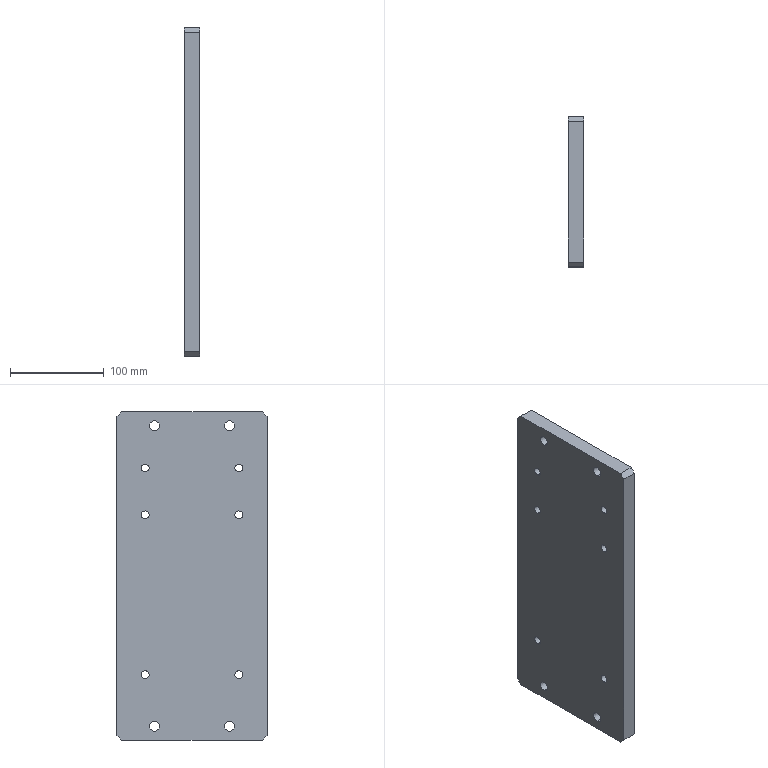Part | SolidWorks | features HoleWzd 2, Chamfer 1, Extrusion 1 | 1 solid | 30 faces | box 16 x 160 x 350 mm | volume 884211 mm3 | cylinder 20 | plane 10 | commonest cylinder face diameters 8.5 x12 10.5 x8
STEP:
#1=CARTESIAN_POINT('',(16.,40.,-165.25));
#2=VERTEX_POINT('',#1);
#3=CARTESIAN_POINT('',(16.,40.,-154.75));
#4=VERTEX_POINT('',#3);
#5=CARTESIAN_POINT('',(16.,40.,-160.));
#6=DIRECTION('',(-1.,0.,0.));
#7=DIRECTION('',(0.,0.,1.));
#8=AXIS2_PLACEMENT_3D('',#5,#6,#7);
#9=CIRCLE('',#8,5.25);
#10=EDGE_CURVE('',#2,#4,#9,.T.);
#11=ORIENTED_EDGE('',*,*,#10,.F.);
#12=CARTESIAN_POINT('',(0.,40.,-165.25));
#13=VERTEX_POINT('',#12);
#14=CARTESIAN_POINT('',(0.,40.,-165.25));
#15=DIRECTION('',(-1.,0.,0.));
#16=VECTOR('',#15,1000.);
#17=LINE('',#14,#16);
#18=EDGE_CURVE('',#2,#13,#17,.T.);
#19=ORIENTED_EDGE('',*,*,#18,.T.);
#20=CARTESIAN_POINT('',(0.,40.,-154.75));
#21=VERTEX_POINT('',#20);
#22=CARTESIAN_POINT('',(0.,40.,-160.));
#23=DIRECTION('',(-1.,0.,0.));
#24=DIRECTION('',(0.,0.,1.));
#25=AXIS2_PLACEMENT_3D('',#22,#23,#24);
#26=CIRCLE('',#25,5.25);
#27=EDGE_CURVE('',#13,#21,#26,.T.);
#28=ORIENTED_EDGE('',*,*,#27,.T.);
#29=CARTESIAN_POINT('',(0.,40.,-154.75));
#30=DIRECTION('',(-1.,0.,0.));
#31=VECTOR('',#30,1000.);
#32=LINE('',#29,#31);
#33=EDGE_CURVE('',#4,#21,#32,.T.);
#34=ORIENTED_EDGE('',*,*,#33,.F.);
#35=EDGE_LOOP('',(#11,#19,#28,#34));
#36=FACE_OUTER_BOUND('',#35,.T.);
#37=CARTESIAN_POINT('',(0.,40.,-160.));
#38=DIRECTION('',(-1.,0.,0.));
#39=DIRECTION('',(0.,0.,1.));
#40=AXIS2_PLACEMENT_3D('',#37,#38,#39);
#41=CYLINDRICAL_SURFACE('',#40,5.25);
#42=ADVANCED_FACE('',(#36),#41,.F.);
#43=CARTESIAN_POINT('',(16.,-40.,-165.25));
#44=VERTEX_POINT('',#43);
#45=CARTESIAN_POINT('',(16.,-40.,-154.75));
#46=VERTEX_POINT('',#45);
#47=CARTESIAN_POINT('',(16.,-40.,-160.));
#48=DIRECTION('',(-1.,0.,0.));
#49=DIRECTION('',(0.,0.,1.));
#50=AXIS2_PLACEMENT_3D('',#47,#48,#49);
#51=CIRCLE('',#50,5.25);
#52=EDGE_CURVE('',#44,#46,#51,.T.);
#53=ORIENTED_EDGE('',*,*,#52,.F.);
#54=CARTESIAN_POINT('',(0.,-40.,-165.25));
#55=VERTEX_POINT('',#54);
#56=CARTESIAN_POINT('',(0.,-40.,-165.25));
#57=DIRECTION('',(-1.,0.,0.));
#58=VECTOR('',#57,1000.);
#59=LINE('',#56,#58);
#60=EDGE_CURVE('',#44,#55,#59,.T.);
#61=ORIENTED_EDGE('',*,*,#60,.T.);
#62=CARTESIAN_POINT('',(0.,-40.,-154.75));
#63=VERTEX_POINT('',#62);
#64=CARTESIAN_POINT('',(0.,-40.,-160.));
#65=DIRECTION('',(-1.,0.,0.));
#66=DIRECTION('',(0.,0.,1.));
#67=AXIS2_PLACEMENT_3D('',#64,#65,#66);
#68=CIRCLE('',#67,5.25);
#69=EDGE_CURVE('',#55,#63,#68,.T.);
#70=ORIENTED_EDGE('',*,*,#69,.T.);
#71=CARTESIAN_POINT('',(0.,-40.,-154.75));
#72=DIRECTION('',(-1.,0.,0.));
#73=VECTOR('',#72,1000.);
#74=LINE('',#71,#73);
#75=EDGE_CURVE('',#46,#63,#74,.T.);
#76=ORIENTED_EDGE('',*,*,#75,.F.);
#77=EDGE_LOOP('',(#53,#61,#70,#76));
#78=FACE_OUTER_BOUND('',#77,.T.);
#79=CARTESIAN_POINT('',(0.,-40.,-160.));
#80=DIRECTION('',(-1.,0.,0.));
#81=DIRECTION('',(0.,0.,1.));
#82=AXIS2_PLACEMENT_3D('',#79,#80,#81);
#83=CYLINDRICAL_SURFACE('',#82,5.25);
#84=ADVANCED_FACE('',(#78),#83,.F.);
#85=CARTESIAN_POINT('',(16.,40.,154.75));
#86=VERTEX_POINT('',#85);
#87=CARTESIAN_POINT('',(16.,40.,165.25));
#88=VERTEX_POINT('',#87);
#89=CARTESIAN_POINT('',(16.,40.,160.));
#90=DIRECTION('',(-1.,0.,0.));
#91=DIRECTION('',(0.,0.,1.));
#92=AXIS2_PLACEMENT_3D('',#89,#90,#91);
#93=CIRCLE('',#92,5.25);
#94=EDGE_CURVE('',#86,#88,#93,.T.);
#95=ORIENTED_EDGE('',*,*,#94,.F.);
#96=CARTESIAN_POINT('',(0.,40.,154.75));
#97=VERTEX_POINT('',#96);
#98=CARTESIAN_POINT('',(0.,40.,154.75));
#99=DIRECTION('',(-1.,0.,0.));
#100=VECTOR('',#99,1000.);
#101=LINE('',#98,#100);
#102=EDGE_CURVE('',#86,#97,#101,.T.);
#103=ORIENTED_EDGE('',*,*,#102,.T.);
#104=CARTESIAN_POINT('',(0.,40.,165.25));
#105=VERTEX_POINT('',#104);
#106=CARTESIAN_POINT('',(0.,40.,160.));
#107=DIRECTION('',(-1.,0.,0.));
#108=DIRECTION('',(0.,0.,1.));
#109=AXIS2_PLACEMENT_3D('',#106,#107,#108);
#110=CIRCLE('',#109,5.25);
#111=EDGE_CURVE('',#97,#105,#110,.T.);
#112=ORIENTED_EDGE('',*,*,#111,.T.);
#113=CARTESIAN_POINT('',(0.,40.,165.25));
#114=DIRECTION('',(-1.,0.,0.));
#115=VECTOR('',#114,1000.);
#116=LINE('',#113,#115);
#117=EDGE_CURVE('',#88,#105,#116,.T.);
#118=ORIENTED_EDGE('',*,*,#117,.F.);
#119=EDGE_LOOP('',(#95,#103,#112,#118));
#120=FACE_OUTER_BOUND('',#119,.T.);
#121=CARTESIAN_POINT('',(0.,40.,160.));
#122=DIRECTION('',(-1.,0.,0.));
#123=DIRECTION('',(0.,0.,1.));
#124=AXIS2_PLACEMENT_3D('',#121,#122,#123);
#125=CYLINDRICAL_SURFACE('',#124,5.25);
#126=ADVANCED_FACE('',(#120),#125,.F.);
#127=CARTESIAN_POINT('',(16.,-40.,154.75));
#128=VERTEX_POINT('',#127);
#129=CARTESIAN_POINT('',(16.,-40.,165.25));
#130=VERTEX_POINT('',#129);
#131=CARTESIAN_POINT('',(16.,-40.,160.));
#132=DIRECTION('',(-1.,0.,0.));
#133=DIRECTION('',(0.,0.,1.));
#134=AXIS2_PLACEMENT_3D('',#131,#132,#133);
#135=CIRCLE('',#134,5.25);
#136=EDGE_CURVE('',#128,#130,#135,.T.);
#137=ORIENTED_EDGE('',*,*,#136,.F.);
#138=CARTESIAN_POINT('',(0.,-40.,154.75));
#139=VERTEX_POINT('',#138);
#140=CARTESIAN_POINT('',(0.,-40.,154.75));
#141=DIRECTION('',(-1.,0.,0.));
#142=VECTOR('',#141,1000.);
#143=LINE('',#140,#142);
#144=EDGE_CURVE('',#128,#139,#143,.T.);
#145=ORIENTED_EDGE('',*,*,#144,.T.);
#146=CARTESIAN_POINT('',(0.,-40.,165.25));
#147=VERTEX_POINT('',#146);
#148=CARTESIAN_POINT('',(0.,-40.,160.));
#149=DIRECTION('',(-1.,0.,0.));
#150=DIRECTION('',(0.,0.,1.));
#151=AXIS2_PLACEMENT_3D('',#148,#149,#150);
#152=CIRCLE('',#151,5.25);
#153=EDGE_CURVE('',#139,#147,#152,.T.);
#154=ORIENTED_EDGE('',*,*,#153,.T.);
#155=CARTESIAN_POINT('',(0.,-40.,165.25));
#156=DIRECTION('',(-1.,0.,0.));
#157=VECTOR('',#156,1000.);
#158=LINE('',#155,#157);
#159=EDGE_CURVE('',#130,#147,#158,.T.);
#160=ORIENTED_EDGE('',*,*,#159,.F.);
#161=EDGE_LOOP('',(#137,#145,#154,#160));
#162=FACE_OUTER_BOUND('',#161,.T.);
#163=CARTESIAN_POINT('',(0.,-40.,160.));
#164=DIRECTION('',(-1.,0.,0.));
#165=DIRECTION('',(0.,0.,1.));
#166=AXIS2_PLACEMENT_3D('',#163,#164,#165);
#167=CYLINDRICAL_SURFACE('',#166,5.25);
#168=ADVANCED_FACE('',(#162),#167,.F.);
#169=CARTESIAN_POINT('',(0.,50.,119.25));
#170=VERTEX_POINT('',#169);
#171=CARTESIAN_POINT('',(0.,50.,110.75));
#172=VERTEX_POINT('',#171);
#173=CARTESIAN_POINT('',(0.,50.,115.));
#174=DIRECTION('',(1.,0.,0.));
#175=DIRECTION('',(0.,0.,-1.));
#176=AXIS2_PLACEMENT_3D('',#173,#174,#175);
#177=CIRCLE('',#176,4.25);
#178=EDGE_CURVE('',#170,#172,#177,.T.);
#179=ORIENTED_EDGE('',*,*,#178,.F.);
#180=CARTESIAN_POINT('',(16.,50.,119.25));
#181=VERTEX_POINT('',#180);
#182=CARTESIAN_POINT('',(16.,50.,119.25));
#183=DIRECTION('',(1.,0.,0.));
#184=VECTOR('',#183,1000.);
#185=LINE('',#182,#184);
#186=EDGE_CURVE('',#170,#181,#185,.T.);
#187=ORIENTED_EDGE('',*,*,#186,.T.);
#188=CARTESIAN_POINT('',(16.,50.,110.75));
#189=VERTEX_POINT('',#188);
#190=CARTESIAN_POINT('',(16.,50.,115.));
#191=DIRECTION('',(1.,0.,0.));
#192=DIRECTION('',(0.,0.,-1.));
#193=AXIS2_PLACEMENT_3D('',#190,#191,#192);
#194=CIRCLE('',#193,4.25);
#195=EDGE_CURVE('',#181,#189,#194,.T.);
#196=ORIENTED_EDGE('',*,*,#195,.T.);
#197=CARTESIAN_POINT('',(16.,50.,110.75));
#198=DIRECTION('',(1.,0.,0.));
#199=VECTOR('',#198,1000.);
#200=LINE('',#197,#199);
#201=EDGE_CURVE('',#172,#189,#200,.T.);
#202=ORIENTED_EDGE('',*,*,#201,.F.);
#203=EDGE_LOOP('',(#179,#187,#196,#202));
#204=FACE_OUTER_BOUND('',#203,.T.);
#205=CARTESIAN_POINT('',(16.,50.,115.));
#206=DIRECTION('',(1.,0.,0.));
#207=DIRECTION('',(0.,0.,-1.));
#208=AXIS2_PLACEMENT_3D('',#205,#206,#207);
#209=CYLINDRICAL_SURFACE('',#208,4.25);
#210=ADVANCED_FACE('',(#204),#209,.F.);
#211=CARTESIAN_POINT('',(0.,-50.,119.25));
#212=VERTEX_POINT('',#211);
#213=CARTESIAN_POINT('',(0.,-50.,110.75));
#214=VERTEX_POINT('',#213);
#215=CARTESIAN_POINT('',(0.,-50.,115.));
#216=DIRECTION('',(1.,0.,0.));
#217=DIRECTION('',(0.,0.,-1.));
#218=AXIS2_PLACEMENT_3D('',#215,#216,#217);
#219=CIRCLE('',#218,4.25);
#220=EDGE_CURVE('',#212,#214,#219,.T.);
#221=ORIENTED_EDGE('',*,*,#220,.F.);
#222=CARTESIAN_POINT('',(16.,-50.,119.25));
#223=VERTEX_POINT('',#222);
#224=CARTESIAN_POINT('',(16.,-50.,119.25));
#225=DIRECTION('',(1.,0.,0.));
#226=VECTOR('',#225,1000.);
#227=LINE('',#224,#226);
#228=EDGE_CURVE('',#212,#223,#227,.T.);
#229=ORIENTED_EDGE('',*,*,#228,.T.);
#230=CARTESIAN_POINT('',(16.,-50.,110.75));
#231=VERTEX_POINT('',#230);
#232=CARTESIAN_POINT('',(16.,-50.,115.));
#233=DIRECTION('',(1.,0.,0.));
#234=DIRECTION('',(0.,0.,-1.));
#235=AXIS2_PLACEMENT_3D('',#232,#233,#234);
#236=CIRCLE('',#235,4.25);
#237=EDGE_CURVE('',#223,#231,#236,.T.);
#238=ORIENTED_EDGE('',*,*,#237,.T.);
#239=CARTESIAN_POINT('',(16.,-50.,110.75));
#240=DIRECTION('',(1.,0.,0.));
#241=VECTOR('',#240,1000.);
#242=LINE('',#239,#241);
#243=EDGE_CURVE('',#214,#231,#242,.T.);
#244=ORIENTED_EDGE('',*,*,#243,.F.);
#245=EDGE_LOOP('',(#221,#229,#238,#244));
#246=FACE_OUTER_BOUND('',#245,.T.);
#247=CARTESIAN_POINT('',(16.,-50.,115.));
#248=DIRECTION('',(1.,0.,0.));
#249=DIRECTION('',(0.,0.,-1.));
#250=AXIS2_PLACEMENT_3D('',#247,#248,#249);
#251=CYLINDRICAL_SURFACE('',#250,4.25);
#252=ADVANCED_FACE('',(#246),#251,.F.);
#253=CARTESIAN_POINT('',(0.,50.,-100.75));
#254=VERTEX_POINT('',#253);
#255=CARTESIAN_POINT('',(0.,50.,-109.25));
#256=VERTEX_POINT('',#255);
#257=CARTESIAN_POINT('',(0.,50.,-105.));
#258=DIRECTION('',(1.,0.,0.));
#259=DIRECTION('',(0.,0.,-1.));
#260=AXIS2_PLACEMENT_3D('',#257,#258,#259);
#261=CIRCLE('',#260,4.25);
#262=EDGE_CURVE('',#254,#256,#261,.T.);
#263=ORIENTED_EDGE('',*,*,#262,.F.);
#264=CARTESIAN_POINT('',(16.,50.,-100.75));
#265=VERTEX_POINT('',#264);
#266=CARTESIAN_POINT('',(16.,50.,-100.75));
#267=DIRECTION('',(1.,0.,0.));
#268=VECTOR('',#267,1000.);
#269=LINE('',#266,#268);
#270=EDGE_CURVE('',#254,#265,#269,.T.);
#271=ORIENTED_EDGE('',*,*,#270,.T.);
#272=CARTESIAN_POINT('',(16.,50.,-109.25));
#273=VERTEX_POINT('',#272);
#274=CARTESIAN_POINT('',(16.,50.,-105.));
#275=DIRECTION('',(1.,0.,0.));
#276=DIRECTION('',(0.,0.,-1.));
#277=AXIS2_PLACEMENT_3D('',#274,#275,#276);
#278=CIRCLE('',#277,4.25);
#279=EDGE_CURVE('',#265,#273,#278,.T.);
#280=ORIENTED_EDGE('',*,*,#279,.T.);
#281=CARTESIAN_POINT('',(16.,50.,-109.25));
#282=DIRECTION('',(1.,0.,0.));
#283=VECTOR('',#282,1000.);
#284=LINE('',#281,#283);
#285=EDGE_CURVE('',#256,#273,#284,.T.);
#286=ORIENTED_EDGE('',*,*,#285,.F.);
#287=EDGE_LOOP('',(#263,#271,#280,#286));
#288=FACE_OUTER_BOUND('',#287,.T.);
#289=CARTESIAN_POINT('',(16.,50.,-105.));
#290=DIRECTION('',(1.,0.,0.));
#291=DIRECTION('',(0.,0.,-1.));
#292=AXIS2_PLACEMENT_3D('',#289,#290,#291);
#293=CYLINDRICAL_SURFACE('',#292,4.25);
#294=ADVANCED_FACE('',(#288),#293,.F.);
#295=CARTESIAN_POINT('',(0.,-50.,-100.75));
#296=VERTEX_POINT('',#295);
#297=CARTESIAN_POINT('',(0.,-50.,-109.25));
#298=VERTEX_POINT('',#297);
#299=CARTESIAN_POINT('',(0.,-50.,-105.));
#300=DIRECTION('',(1.,0.,0.));
#301=DIRECTION('',(0.,0.,-1.));
#302=AXIS2_PLACEMENT_3D('',#299,#300,#301);
#303=CIRCLE('',#302,4.25);
#304=EDGE_CURVE('',#296,#298,#303,.T.);
#305=ORIENTED_EDGE('',*,*,#304,.F.);
#306=CARTESIAN_POINT('',(16.,-50.,-100.75));
#307=VERTEX_POINT('',#306);
#308=CARTESIAN_POINT('',(16.,-50.,-100.75));
#309=DIRECTION('',(1.,0.,0.));
#310=VECTOR('',#309,1000.);
#311=LINE('',#308,#310);
#312=EDGE_CURVE('',#296,#307,#311,.T.);
#313=ORIENTED_EDGE('',*,*,#312,.T.);
#314=CARTESIAN_POINT('',(16.,-50.,-109.25));
#315=VERTEX_POINT('',#314);
#316=CARTESIAN_POINT('',(16.,-50.,-105.));
#317=DIRECTION('',(1.,0.,0.));
#318=DIRECTION('',(0.,0.,-1.));
#319=AXIS2_PLACEMENT_3D('',#316,#317,#318);
#320=CIRCLE('',#319,4.25);
#321=EDGE_CURVE('',#307,#315,#320,.T.);
#322=ORIENTED_EDGE('',*,*,#321,.T.);
#323=CARTESIAN_POINT('',(16.,-50.,-109.25));
#324=DIRECTION('',(1.,0.,0.));
#325=VECTOR('',#324,1000.);
#326=LINE('',#323,#325);
#327=EDGE_CURVE('',#298,#315,#326,.T.);
#328=ORIENTED_EDGE('',*,*,#327,.F.);
#329=EDGE_LOOP('',(#305,#313,#322,#328));
#330=FACE_OUTER_BOUND('',#329,.T.);
#331=CARTESIAN_POINT('',(16.,-50.,-105.));
#332=DIRECTION('',(1.,0.,0.));
#333=DIRECTION('',(0.,0.,-1.));
#334=AXIS2_PLACEMENT_3D('',#331,#332,#333);
#335=CYLINDRICAL_SURFACE('',#334,4.25);
#336=ADVANCED_FACE('',(#330),#335,.F.);
#337=CARTESIAN_POINT('',(0.,50.,69.25));
#338=VERTEX_POINT('',#337);
#339=CARTESIAN_POINT('',(0.,50.,60.75));
#340=VERTEX_POINT('',#339);
#341=CARTESIAN_POINT('',(0.,50.,65.));
#342=DIRECTION('',(1.,0.,0.));
#343=DIRECTION('',(0.,0.,-1.));
#344=AXIS2_PLACEMENT_3D('',#341,#342,#343);
#345=CIRCLE('',#344,4.25);
#346=EDGE_CURVE('',#338,#340,#345,.T.);
#347=ORIENTED_EDGE('',*,*,#346,.F.);
#348=CARTESIAN_POINT('',(16.,50.,69.25));
#349=VERTEX_POINT('',#348);
#350=CARTESIAN_POINT('',(16.,50.,69.25));
#351=DIRECTION('',(1.,0.,0.));
#352=VECTOR('',#351,1000.);
#353=LINE('',#350,#352);
#354=EDGE_CURVE('',#338,#349,#353,.T.);
#355=ORIENTED_EDGE('',*,*,#354,.T.);
#356=CARTESIAN_POINT('',(16.,50.,60.75));
#357=VERTEX_POINT('',#356);
#358=CARTESIAN_POINT('',(16.,50.,65.));
#359=DIRECTION('',(1.,0.,0.));
#360=DIRECTION('',(0.,0.,-1.));
#361=AXIS2_PLACEMENT_3D('',#358,#359,#360);
#362=CIRCLE('',#361,4.25);
#363=EDGE_CURVE('',#349,#357,#362,.T.);
#364=ORIENTED_EDGE('',*,*,#363,.T.);
#365=CARTESIAN_POINT('',(16.,50.,60.75));
#366=DIRECTION('',(1.,0.,0.));
#367=VECTOR('',#366,1000.);
#368=LINE('',#365,#367);
#369=EDGE_CURVE('',#340,#357,#368,.T.);
#370=ORIENTED_EDGE('',*,*,#369,.F.);
#371=EDGE_LOOP('',(#347,#355,#364,#370));
#372=FACE_OUTER_BOUND('',#371,.T.);
#373=CARTESIAN_POINT('',(16.,50.,65.));
#374=DIRECTION('',(1.,0.,0.));
#375=DIRECTION('',(0.,0.,-1.));
#376=AXIS2_PLACEMENT_3D('',#373,#374,#375);
#377=CYLINDRICAL_SURFACE('',#376,4.25);
#378=ADVANCED_FACE('',(#372),#377,.F.);
#379=CARTESIAN_POINT('',(0.,-50.,69.25));
#380=VERTEX_POINT('',#379);
#381=CARTESIAN_POINT('',(0.,-50.,60.75));
#382=VERTEX_POINT('',#381);
#383=CARTESIAN_POINT('',(0.,-50.,65.));
#384=DIRECTION('',(1.,0.,0.));
#385=DIRECTION('',(0.,0.,-1.));
#386=AXIS2_PLACEMENT_3D('',#383,#384,#385);
#387=CIRCLE('',#386,4.25);
#388=EDGE_CURVE('',#380,#382,#387,.T.);
#389=ORIENTED_EDGE('',*,*,#388,.F.);
#390=CARTESIAN_POINT('',(16.,-50.,69.25));
#391=VERTEX_POINT('',#390);
#392=CARTESIAN_POINT('',(16.,-50.,69.25));
#393=DIRECTION('',(1.,0.,0.));
#394=VECTOR('',#393,1000.);
#395=LINE('',#392,#394);
#396=EDGE_CURVE('',#380,#391,#395,.T.);
#397=ORIENTED_EDGE('',*,*,#396,.T.);
#398=CARTESIAN_POINT('',(16.,-50.,60.75));
#399=VERTEX_POINT('',#398);
#400=CARTESIAN_POINT('',(16.,-50.,65.));
#401=DIRECTION('',(1.,0.,0.));
#402=DIRECTION('',(0.,0.,-1.));
#403=AXIS2_PLACEMENT_3D('',#400,#401,#402);
#404=CIRCLE('',#403,4.25);
#405=EDGE_CURVE('',#391,#399,#404,.T.);
#406=ORIENTED_EDGE('',*,*,#405,.T.);
#407=CARTESIAN_POINT('',(16.,-50.,60.75));
#408=DIRECTION('',(1.,0.,0.));
#409=VECTOR('',#408,1000.);
#410=LINE('',#407,#409);
#411=EDGE_CURVE('',#382,#399,#410,.T.);
#412=ORIENTED_EDGE('',*,*,#411,.F.);
#413=EDGE_LOOP('',(#389,#397,#406,#412));
#414=FACE_OUTER_BOUND('',#413,.T.);
#415=CARTESIAN_POINT('',(16.,-50.,65.));
#416=DIRECTION('',(1.,0.,0.));
#417=DIRECTION('',(0.,0.,-1.));
#418=AXIS2_PLACEMENT_3D('',#415,#416,#417);
#419=CYLINDRICAL_SURFACE('',#418,4.25);
#420=ADVANCED_FACE('',(#414),#419,.F.);
#421=CARTESIAN_POINT('',(0.,40.,-160.));
#422=DIRECTION('',(-1.,0.,0.));
#423=DIRECTION('',(0.,0.,1.));
#424=AXIS2_PLACEMENT_3D('',#421,#422,#423);
#425=CIRCLE('',#424,5.25);
#426=EDGE_CURVE('',#21,#13,#425,.T.);
#427=ORIENTED_EDGE('',*,*,#426,.F.);
#428=ORIENTED_EDGE('',*,*,#27,.F.);
#429=EDGE_LOOP('',(#427,#428));
#430=FACE_BOUND('',#429,.T.);
#431=CARTESIAN_POINT('',(0.,-40.,-160.));
#432=DIRECTION('',(-1.,0.,0.));
#433=DIRECTION('',(0.,0.,1.));
#434=AXIS2_PLACEMENT_3D('',#431,#432,#433);
#435=CIRCLE('',#434,5.25);
#436=EDGE_CURVE('',#63,#55,#435,.T.);
#437=ORIENTED_EDGE('',*,*,#436,.F.);
#438=ORIENTED_EDGE('',*,*,#69,.F.);
#439=EDGE_LOOP('',(#437,#438));
#440=FACE_BOUND('',#439,.T.);
#441=CARTESIAN_POINT('',(0.,-40.,160.));
#442=DIRECTION('',(-1.,0.,0.));
#443=DIRECTION('',(0.,0.,1.));
#444=AXIS2_PLACEMENT_3D('',#441,#442,#443);
#445=CIRCLE('',#444,5.25);
#446=EDGE_CURVE('',#147,#139,#445,.T.);
#447=ORIENTED_EDGE('',*,*,#446,.F.);
#448=ORIENTED_EDGE('',*,*,#153,.F.);
#449=EDGE_LOOP('',(#447,#448));
#450=FACE_BOUND('',#449,.T.);
#451=CARTESIAN_POINT('',(0.,50.,115.));
#452=DIRECTION('',(1.,0.,0.));
#453=DIRECTION('',(0.,0.,-1.));
#454=AXIS2_PLACEMENT_3D('',#451,#452,#453);
#455=CIRCLE('',#454,4.25);
#456=EDGE_CURVE('',#172,#170,#455,.T.);
#457=ORIENTED_EDGE('',*,*,#456,.T.);
#458=ORIENTED_EDGE('',*,*,#178,.T.);
#459=EDGE_LOOP('',(#457,#458));
#460=FACE_BOUND('',#459,.T.);
#461=CARTESIAN_POINT('',(0.,-50.,115.));
#462=DIRECTION('',(1.,0.,0.));
#463=DIRECTION('',(0.,0.,-1.));
#464=AXIS2_PLACEMENT_3D('',#461,#462,#463);
#465=CIRCLE('',#464,4.25);
#466=EDGE_CURVE('',#214,#212,#465,.T.);
#467=ORIENTED_EDGE('',*,*,#466,.T.);
#468=ORIENTED_EDGE('',*,*,#220,.T.);
#469=EDGE_LOOP('',(#467,#468));
#470=FACE_BOUND('',#469,.T.);
#471=CARTESIAN_POINT('',(0.,50.,-105.));
#472=DIRECTION('',(1.,0.,0.));
#473=DIRECTION('',(0.,0.,-1.));
#474=AXIS2_PLACEMENT_3D('',#471,#472,#473);
#475=CIRCLE('',#474,4.25);
#476=EDGE_CURVE('',#256,#254,#475,.T.);
#477=ORIENTED_EDGE('',*,*,#476,.T.);
#478=ORIENTED_EDGE('',*,*,#262,.T.);
#479=EDGE_LOOP('',(#477,#478));
#480=FACE_BOUND('',#479,.T.);
#481=CARTESIAN_POINT('',(0.,-50.,-105.));
#482=DIRECTION('',(1.,0.,0.));
#483=DIRECTION('',(0.,0.,-1.));
#484=AXIS2_PLACEMENT_3D('',#481,#482,#483);
#485=CIRCLE('',#484,4.25);
#486=EDGE_CURVE('',#298,#296,#485,.T.);
#487=ORIENTED_EDGE('',*,*,#486,.T.);
#488=ORIENTED_EDGE('',*,*,#304,.T.);
#489=EDGE_LOOP('',(#487,#488));
#490=FACE_BOUND('',#489,.T.);
#491=CARTESIAN_POINT('',(0.,50.,65.));
#492=DIRECTION('',(1.,0.,0.));
#493=DIRECTION('',(0.,0.,-1.));
#494=AXIS2_PLACEMENT_3D('',#491,#492,#493);
#495=CIRCLE('',#494,4.25);
#496=EDGE_CURVE('',#340,#338,#495,.T.);
#497=ORIENTED_EDGE('',*,*,#496,.T.);
#498=ORIENTED_EDGE('',*,*,#346,.T.);
#499=EDGE_LOOP('',(#497,#498));
#500=FACE_BOUND('',#499,.T.);
#501=CARTESIAN_POINT('',(0.,-50.,65.));
#502=DIRECTION('',(1.,0.,0.));
#503=DIRECTION('',(0.,0.,-1.));
#504=AXIS2_PLACEMENT_3D('',#501,#502,#503);
#505=CIRCLE('',#504,4.25);
#506=EDGE_CURVE('',#382,#380,#505,.T.);
#507=ORIENTED_EDGE('',*,*,#506,.T.);
#508=ORIENTED_EDGE('',*,*,#388,.T.);
#509=EDGE_LOOP('',(#507,#508));
#510=FACE_BOUND('',#509,.T.);
#511=CARTESIAN_POINT('',(0.,75.,175.));
#512=VERTEX_POINT('',#511);
#513=CARTESIAN_POINT('',(0.,-75.,175.));
#514=VERTEX_POINT('',#513);
#515=CARTESIAN_POINT('',(0.,80.,175.));
#516=DIRECTION('',(0.,-1.,0.));
#517=VECTOR('',#516,1000.);
#518=LINE('',#515,#517);
#519=EDGE_CURVE('',#512,#514,#518,.T.);
#520=ORIENTED_EDGE('',*,*,#519,.F.);
#521=CARTESIAN_POINT('',(0.,80.,170.));
#522=VERTEX_POINT('',#521);
#523=CARTESIAN_POINT('',(0.,75.,175.));
#524=DIRECTION('',(0.,0.7071,-0.7071));
#525=VECTOR('',#524,1000.);
#526=LINE('',#523,#525);
#527=EDGE_CURVE('',#512,#522,#526,.T.);
#528=ORIENTED_EDGE('',*,*,#527,.T.);
#529=CARTESIAN_POINT('',(0.,80.,-170.));
#530=VERTEX_POINT('',#529);
#531=CARTESIAN_POINT('',(0.,80.,175.));
#532=DIRECTION('',(0.,0.,1.));
#533=VECTOR('',#532,1000.);
#534=LINE('',#531,#533);
#535=EDGE_CURVE('',#530,#522,#534,.T.);
#536=ORIENTED_EDGE('',*,*,#535,.F.);
#537=CARTESIAN_POINT('',(0.,75.,-175.));
#538=VERTEX_POINT('',#537);
#539=CARTESIAN_POINT('',(0.,80.,-170.));
#540=DIRECTION('',(0.,-0.7071,-0.7071));
#541=VECTOR('',#540,1000.);
#542=LINE('',#539,#541);
#543=EDGE_CURVE('',#530,#538,#542,.T.);
#544=ORIENTED_EDGE('',*,*,#543,.T.);
#545=CARTESIAN_POINT('',(0.,-75.,-175.));
#546=VERTEX_POINT('',#545);
#547=CARTESIAN_POINT('',(0.,80.,-175.));
#548=DIRECTION('',(0.,1.,0.));
#549=VECTOR('',#548,1000.);
#550=LINE('',#547,#549);
#551=EDGE_CURVE('',#546,#538,#550,.T.);
#552=ORIENTED_EDGE('',*,*,#551,.F.);
#553=CARTESIAN_POINT('',(0.,-80.,-170.));
#554=VERTEX_POINT('',#553);
#555=CARTESIAN_POINT('',(0.,-75.,-175.));
#556=DIRECTION('',(0.,-0.7071,0.7071));
#557=VECTOR('',#556,1000.);
#558=LINE('',#555,#557);
#559=EDGE_CURVE('',#546,#554,#558,.T.);
#560=ORIENTED_EDGE('',*,*,#559,.T.);
#561=CARTESIAN_POINT('',(0.,-80.,170.));
#562=VERTEX_POINT('',#561);
#563=CARTESIAN_POINT('',(0.,-80.,175.));
#564=DIRECTION('',(0.,0.,-1.));
#565=VECTOR('',#564,1000.);
#566=LINE('',#563,#565);
#567=EDGE_CURVE('',#562,#554,#566,.T.);
#568=ORIENTED_EDGE('',*,*,#567,.F.);
#569=CARTESIAN_POINT('',(0.,-80.,170.));
#570=DIRECTION('',(0.,0.7071,0.7071));
#571=VECTOR('',#570,1000.);
#572=LINE('',#569,#571);
#573=EDGE_CURVE('',#562,#514,#572,.T.);
#574=ORIENTED_EDGE('',*,*,#573,.T.);
#575=EDGE_LOOP('',(#520,#528,#536,#544,#552,#560,#568,#574));
#576=FACE_OUTER_BOUND('',#575,.T.);
#577=CARTESIAN_POINT('',(0.,40.,160.));
#578=DIRECTION('',(-1.,0.,0.));
#579=DIRECTION('',(0.,0.,1.));
#580=AXIS2_PLACEMENT_3D('',#577,#578,#579);
#581=CIRCLE('',#580,5.25);
#582=EDGE_CURVE('',#105,#97,#581,.T.);
#583=ORIENTED_EDGE('',*,*,#582,.F.);
#584=ORIENTED_EDGE('',*,*,#111,.F.);
#585=EDGE_LOOP('',(#583,#584));
#586=FACE_BOUND('',#585,.T.);
#587=CARTESIAN_POINT('',(0.,0.,0.));
#588=DIRECTION('',(1.,0.,0.));
#589=DIRECTION('',(0.,0.,-1.));
#590=AXIS2_PLACEMENT_3D('',#587,#588,#589);
#591=PLANE('',#590);
#592=ADVANCED_FACE('',(#430,#440,#450,#460,#470,#480,#490,#500,#510,#576,#586),#591,.F.);
#593=ORIENTED_EDGE('',*,*,#551,.T.);
#594=CARTESIAN_POINT('',(16.,75.,-175.));
#595=VERTEX_POINT('',#594);
#596=CARTESIAN_POINT('',(16.,75.,-175.));
#597=DIRECTION('',(1.,0.,0.));
#598=VECTOR('',#597,1000.);
#599=LINE('',#596,#598);
#600=EDGE_CURVE('',#538,#595,#599,.T.);
#601=ORIENTED_EDGE('',*,*,#600,.T.);
#602=CARTESIAN_POINT('',(16.,-75.,-175.));
#603=VERTEX_POINT('',#602);
#604=CARTESIAN_POINT('',(16.,80.,-175.));
#605=DIRECTION('',(0.,1.,0.));
#606=VECTOR('',#605,1000.);
#607=LINE('',#604,#606);
#608=EDGE_CURVE('',#603,#595,#607,.T.);
#609=ORIENTED_EDGE('',*,*,#608,.F.);
#610=CARTESIAN_POINT('',(16.,-75.,-175.));
#611=DIRECTION('',(-1.,0.,0.));
#612=VECTOR('',#611,1000.);
#613=LINE('',#610,#612);
#614=EDGE_CURVE('',#603,#546,#613,.T.);
#615=ORIENTED_EDGE('',*,*,#614,.T.);
#616=EDGE_LOOP('',(#593,#601,#609,#615));
#617=FACE_OUTER_BOUND('',#616,.T.);
#618=CARTESIAN_POINT('',(16.,80.,-175.));
#619=DIRECTION('',(0.,0.,1.));
#620=DIRECTION('',(0.,-1.,0.));
#621=AXIS2_PLACEMENT_3D('',#618,#619,#620);
#622=PLANE('',#621);
#623=ADVANCED_FACE('',(#617),#622,.F.);
#624=ORIENTED_EDGE('',*,*,#535,.T.);
#625=CARTESIAN_POINT('',(16.,80.,170.));
#626=VERTEX_POINT('',#625);
#627=CARTESIAN_POINT('',(16.,80.,170.));
#628=DIRECTION('',(1.,0.,0.));
#629=VECTOR('',#628,1000.);
#630=LINE('',#627,#629);
#631=EDGE_CURVE('',#522,#626,#630,.T.);
#632=ORIENTED_EDGE('',*,*,#631,.T.);
#633=CARTESIAN_POINT('',(16.,80.,-170.));
#634=VERTEX_POINT('',#633);
#635=CARTESIAN_POINT('',(16.,80.,175.));
#636=DIRECTION('',(0.,0.,1.));
#637=VECTOR('',#636,1000.);
#638=LINE('',#635,#637);
#639=EDGE_CURVE('',#634,#626,#638,.T.);
#640=ORIENTED_EDGE('',*,*,#639,.F.);
#641=CARTESIAN_POINT('',(16.,80.,-170.));
#642=DIRECTION('',(-1.,0.,0.));
#643=VECTOR('',#642,1000.);
#644=LINE('',#641,#643);
#645=EDGE_CURVE('',#634,#530,#644,.T.);
#646=ORIENTED_EDGE('',*,*,#645,.T.);
#647=EDGE_LOOP('',(#624,#632,#640,#646));
#648=FACE_OUTER_BOUND('',#647,.T.);
#649=CARTESIAN_POINT('',(16.,80.,175.));
#650=DIRECTION('',(0.,-1.,0.));
#651=DIRECTION('',(0.,0.,-1.));
#652=AXIS2_PLACEMENT_3D('',#649,#650,#651);
#653=PLANE('',#652);
#654=ADVANCED_FACE('',(#648),#653,.F.);
#655=CARTESIAN_POINT('',(16.,75.,175.));
#656=VERTEX_POINT('',#655);
#657=CARTESIAN_POINT('',(16.,-75.,175.));
#658=VERTEX_POINT('',#657);
#659=CARTESIAN_POINT('',(16.,80.,175.));
#660=DIRECTION('',(0.,-1.,0.));
#661=VECTOR('',#660,1000.);
#662=LINE('',#659,#661);
#663=EDGE_CURVE('',#656,#658,#662,.T.);
#664=ORIENTED_EDGE('',*,*,#663,.F.);
#665=CARTESIAN_POINT('',(16.,75.,175.));
#666=DIRECTION('',(-1.,0.,0.));
#667=VECTOR('',#666,1000.);
#668=LINE('',#665,#667);
#669=EDGE_CURVE('',#656,#512,#668,.T.);
#670=ORIENTED_EDGE('',*,*,#669,.T.);
#671=ORIENTED_EDGE('',*,*,#519,.T.);
#672=CARTESIAN_POINT('',(16.,-75.,175.));
#673=DIRECTION('',(1.,0.,0.));
#674=VECTOR('',#673,1000.);
#675=LINE('',#672,#674);
#676=EDGE_CURVE('',#514,#658,#675,.T.);
#677=ORIENTED_EDGE('',*,*,#676,.T.);
#678=EDGE_LOOP('',(#664,#670,#671,#677));
#679=FACE_OUTER_BOUND('',#678,.T.);
#680=CARTESIAN_POINT('',(16.,80.,175.));
#681=DIRECTION('',(0.,0.,-1.));
#682=DIRECTION('',(0.,1.,0.));
#683=AXIS2_PLACEMENT_3D('',#680,#681,#682);
#684=PLANE('',#683);
#685=ADVANCED_FACE('',(#679),#684,.F.);
#686=CARTESIAN_POINT('',(16.,-80.,170.));
#687=VERTEX_POINT('',#686);
#688=CARTESIAN_POINT('',(16.,-80.,-170.));
#689=VERTEX_POINT('',#688);
#690=CARTESIAN_POINT('',(16.,-80.,175.));
#691=DIRECTION('',(0.,0.,-1.));
#692=VECTOR('',#691,1000.);
#693=LINE('',#690,#692);
#694=EDGE_CURVE('',#687,#689,#693,.T.);
#695=ORIENTED_EDGE('',*,*,#694,.F.);
#696=CARTESIAN_POINT('',(16.,-80.,170.));
#697=DIRECTION('',(-1.,0.,0.));
#698=VECTOR('',#697,1000.);
#699=LINE('',#696,#698);
#700=EDGE_CURVE('',#687,#562,#699,.T.);
#701=ORIENTED_EDGE('',*,*,#700,.T.);
#702=ORIENTED_EDGE('',*,*,#567,.T.);
#703=CARTESIAN_POINT('',(16.,-80.,-170.));
#704=DIRECTION('',(1.,0.,0.));
#705=VECTOR('',#704,1000.);
#706=LINE('',#703,#705);
#707=EDGE_CURVE('',#554,#689,#706,.T.);
#708=ORIENTED_EDGE('',*,*,#707,.T.);
#709=EDGE_LOOP('',(#695,#701,#702,#708));
#710=FACE_OUTER_BOUND('',#709,.T.);
#711=CARTESIAN_POINT('',(16.,-80.,175.));
#712=DIRECTION('',(0.,1.,0.));
#713=DIRECTION('',(0.,0.,1.));
#714=AXIS2_PLACEMENT_3D('',#711,#712,#713);
#715=PLANE('',#714);
#716=ADVANCED_FACE('',(#710),#715,.F.);
#717=CARTESIAN_POINT('',(16.,40.,-160.));
#718=DIRECTION('',(-1.,0.,0.));
#719=DIRECTION('',(0.,0.,1.));
#720=AXIS2_PLACEMENT_3D('',#717,#718,#719);
#721=CIRCLE('',#720,5.25);
#722=EDGE_CURVE('',#4,#2,#721,.T.);
#723=ORIENTED_EDGE('',*,*,#722,.T.);
#724=ORIENTED_EDGE('',*,*,#10,.T.);
#725=EDGE_LOOP('',(#723,#724));
#726=FACE_BOUND('',#725,.T.);
#727=CARTESIAN_POINT('',(16.,-40.,-160.));
#728=DIRECTION('',(-1.,0.,0.));
#729=DIRECTION('',(0.,0.,1.));
#730=AXIS2_PLACEMENT_3D('',#727,#728,#729);
#731=CIRCLE('',#730,5.25);
#732=EDGE_CURVE('',#46,#44,#731,.T.);
#733=ORIENTED_EDGE('',*,*,#732,.T.);
#734=ORIENTED_EDGE('',*,*,#52,.T.);
#735=EDGE_LOOP('',(#733,#734));
#736=FACE_BOUND('',#735,.T.);
#737=CARTESIAN_POINT('',(16.,40.,160.));
#738=DIRECTION('',(-1.,0.,0.));
#739=DIRECTION('',(0.,0.,1.));
#740=AXIS2_PLACEMENT_3D('',#737,#738,#739);
#741=CIRCLE('',#740,5.25);
#742=EDGE_CURVE('',#88,#86,#741,.T.);
#743=ORIENTED_EDGE('',*,*,#742,.T.);
#744=ORIENTED_EDGE('',*,*,#94,.T.);
#745=EDGE_LOOP('',(#743,#744));
#746=FACE_BOUND('',#745,.T.);
#747=CARTESIAN_POINT('',(16.,-40.,160.));
#748=DIRECTION('',(-1.,0.,0.));
#749=DIRECTION('',(0.,0.,1.));
#750=AXIS2_PLACEMENT_3D('',#747,#748,#749);
#751=CIRCLE('',#750,5.25);
#752=EDGE_CURVE('',#130,#128,#751,.T.);
#753=ORIENTED_EDGE('',*,*,#752,.T.);
#754=ORIENTED_EDGE('',*,*,#136,.T.);
#755=EDGE_LOOP('',(#753,#754));
#756=FACE_BOUND('',#755,.T.);
#757=CARTESIAN_POINT('',(16.,50.,115.));
#758=DIRECTION('',(1.,0.,0.));
#759=DIRECTION('',(0.,0.,-1.));
#760=AXIS2_PLACEMENT_3D('',#757,#758,#759);
#761=CIRCLE('',#760,4.25);
#762=EDGE_CURVE('',#189,#181,#761,.T.);
#763=ORIENTED_EDGE('',*,*,#762,.F.);
#764=ORIENTED_EDGE('',*,*,#195,.F.);
#765=EDGE_LOOP('',(#763,#764));
#766=FACE_BOUND('',#765,.T.);
#767=CARTESIAN_POINT('',(16.,-50.,115.));
#768=DIRECTION('',(1.,0.,0.));
#769=DIRECTION('',(0.,0.,-1.));
#770=AXIS2_PLACEMENT_3D('',#767,#768,#769);
#771=CIRCLE('',#770,4.25);
#772=EDGE_CURVE('',#231,#223,#771,.T.);
#773=ORIENTED_EDGE('',*,*,#772,.F.);
#774=ORIENTED_EDGE('',*,*,#237,.F.);
#775=EDGE_LOOP('',(#773,#774));
#776=FACE_BOUND('',#775,.T.);
#777=CARTESIAN_POINT('',(16.,50.,-105.));
#778=DIRECTION('',(1.,0.,0.));
#779=DIRECTION('',(0.,0.,-1.));
#780=AXIS2_PLACEMENT_3D('',#777,#778,#779);
#781=CIRCLE('',#780,4.25);
#782=EDGE_CURVE('',#273,#265,#781,.T.);
#783=ORIENTED_EDGE('',*,*,#782,.F.);
#784=ORIENTED_EDGE('',*,*,#279,.F.);
#785=EDGE_LOOP('',(#783,#784));
#786=FACE_BOUND('',#785,.T.);
#787=CARTESIAN_POINT('',(16.,-50.,-105.));
#788=DIRECTION('',(1.,0.,0.));
#789=DIRECTION('',(0.,0.,-1.));
#790=AXIS2_PLACEMENT_3D('',#787,#788,#789);
#791=CIRCLE('',#790,4.25);
#792=EDGE_CURVE('',#315,#307,#791,.T.);
#793=ORIENTED_EDGE('',*,*,#792,.F.);
#794=ORIENTED_EDGE('',*,*,#321,.F.);
#795=EDGE_LOOP('',(#793,#794));
#796=FACE_BOUND('',#795,.T.);
#797=CARTESIAN_POINT('',(16.,50.,65.));
#798=DIRECTION('',(1.,0.,0.));
#799=DIRECTION('',(0.,0.,-1.));
#800=AXIS2_PLACEMENT_3D('',#797,#798,#799);
#801=CIRCLE('',#800,4.25);
#802=EDGE_CURVE('',#357,#349,#801,.T.);
#803=ORIENTED_EDGE('',*,*,#802,.F.);
#804=ORIENTED_EDGE('',*,*,#363,.F.);
#805=EDGE_LOOP('',(#803,#804));
#806=FACE_BOUND('',#805,.T.);
#807=CARTESIAN_POINT('',(16.,-50.,65.));
#808=DIRECTION('',(1.,0.,0.));
#809=DIRECTION('',(0.,0.,-1.));
#810=AXIS2_PLACEMENT_3D('',#807,#808,#809);
#811=CIRCLE('',#810,4.25);
#812=EDGE_CURVE('',#399,#391,#811,.T.);
#813=ORIENTED_EDGE('',*,*,#812,.F.);
#814=ORIENTED_EDGE('',*,*,#405,.F.);
#815=EDGE_LOOP('',(#813,#814));
#816=FACE_BOUND('',#815,.T.);
#817=ORIENTED_EDGE('',*,*,#639,.T.);
#818=CARTESIAN_POINT('',(16.,125.,125.));
#819=DIRECTION('',(0.,-0.7071,0.7071));
#820=VECTOR('',#819,1000.);
#821=LINE('',#818,#820);
#822=EDGE_CURVE('',#626,#656,#821,.T.);
#823=ORIENTED_EDGE('',*,*,#822,.T.);
#824=ORIENTED_EDGE('',*,*,#663,.T.);
#825=CARTESIAN_POINT('',(16.,-125.,125.));
#826=DIRECTION('',(0.,-0.7071,-0.7071));
#827=VECTOR('',#826,1000.);
#828=LINE('',#825,#827);
#829=EDGE_CURVE('',#658,#687,#828,.T.);
#830=ORIENTED_EDGE('',*,*,#829,.T.);
#831=ORIENTED_EDGE('',*,*,#694,.T.);
#832=CARTESIAN_POINT('',(16.,-125.,-125.));
#833=DIRECTION('',(0.,0.7071,-0.7071));
#834=VECTOR('',#833,1000.);
#835=LINE('',#832,#834);
#836=EDGE_CURVE('',#689,#603,#835,.T.);
#837=ORIENTED_EDGE('',*,*,#836,.T.);
#838=ORIENTED_EDGE('',*,*,#608,.T.);
#839=CARTESIAN_POINT('',(16.,125.,-125.));
#840=DIRECTION('',(0.,0.7071,0.7071));
#841=VECTOR('',#840,1000.);
#842=LINE('',#839,#841);
#843=EDGE_CURVE('',#595,#634,#842,.T.);
#844=ORIENTED_EDGE('',*,*,#843,.T.);
#845=EDGE_LOOP('',(#817,#823,#824,#830,#831,#837,#838,#844));
#846=FACE_OUTER_BOUND('',#845,.T.);
#847=CARTESIAN_POINT('',(16.,0.,0.));
#848=DIRECTION('',(1.,0.,0.));
#849=DIRECTION('',(0.,0.,-1.));
#850=AXIS2_PLACEMENT_3D('',#847,#848,#849);
#851=PLANE('',#850);
#852=ADVANCED_FACE('',(#726,#736,#746,#756,#766,#776,#786,#796,#806,#816,#846),#851,.T.);
#853=ORIENTED_EDGE('',*,*,#396,.F.);
#854=ORIENTED_EDGE('',*,*,#506,.F.);
#855=ORIENTED_EDGE('',*,*,#411,.T.);
#856=ORIENTED_EDGE('',*,*,#812,.T.);
#857=EDGE_LOOP('',(#853,#854,#855,#856));
#858=FACE_OUTER_BOUND('',#857,.T.);
#859=CARTESIAN_POINT('',(16.,-50.,65.));
#860=DIRECTION('',(1.,0.,0.));
#861=DIRECTION('',(0.,0.,-1.));
#862=AXIS2_PLACEMENT_3D('',#859,#860,#861);
#863=CYLINDRICAL_SURFACE('',#862,4.25);
#864=ADVANCED_FACE('',(#858),#863,.F.);
#865=ORIENTED_EDGE('',*,*,#354,.F.);
#866=ORIENTED_EDGE('',*,*,#496,.F.);
#867=ORIENTED_EDGE('',*,*,#369,.T.);
#868=ORIENTED_EDGE('',*,*,#802,.T.);
#869=EDGE_LOOP('',(#865,#866,#867,#868));
#870=FACE_OUTER_BOUND('',#869,.T.);
#871=CARTESIAN_POINT('',(16.,50.,65.));
#872=DIRECTION('',(1.,0.,0.));
#873=DIRECTION('',(0.,0.,-1.));
#874=AXIS2_PLACEMENT_3D('',#871,#872,#873);
#875=CYLINDRICAL_SURFACE('',#874,4.25);
#876=ADVANCED_FACE('',(#870),#875,.F.);
#877=ORIENTED_EDGE('',*,*,#312,.F.);
#878=ORIENTED_EDGE('',*,*,#486,.F.);
#879=ORIENTED_EDGE('',*,*,#327,.T.);
#880=ORIENTED_EDGE('',*,*,#792,.T.);
#881=EDGE_LOOP('',(#877,#878,#879,#880));
#882=FACE_OUTER_BOUND('',#881,.T.);
#883=CARTESIAN_POINT('',(16.,-50.,-105.));
#884=DIRECTION('',(1.,0.,0.));
#885=DIRECTION('',(0.,0.,-1.));
#886=AXIS2_PLACEMENT_3D('',#883,#884,#885);
#887=CYLINDRICAL_SURFACE('',#886,4.25);
#888=ADVANCED_FACE('',(#882),#887,.F.);
#889=ORIENTED_EDGE('',*,*,#270,.F.);
#890=ORIENTED_EDGE('',*,*,#476,.F.);
#891=ORIENTED_EDGE('',*,*,#285,.T.);
#892=ORIENTED_EDGE('',*,*,#782,.T.);
#893=EDGE_LOOP('',(#889,#890,#891,#892));
#894=FACE_OUTER_BOUND('',#893,.T.);
#895=CARTESIAN_POINT('',(16.,50.,-105.));
#896=DIRECTION('',(1.,0.,0.));
#897=DIRECTION('',(0.,0.,-1.));
#898=AXIS2_PLACEMENT_3D('',#895,#896,#897);
#899=CYLINDRICAL_SURFACE('',#898,4.25);
#900=ADVANCED_FACE('',(#894),#899,.F.);
#901=ORIENTED_EDGE('',*,*,#228,.F.);
#902=ORIENTED_EDGE('',*,*,#466,.F.);
#903=ORIENTED_EDGE('',*,*,#243,.T.);
#904=ORIENTED_EDGE('',*,*,#772,.T.);
#905=EDGE_LOOP('',(#901,#902,#903,#904));
#906=FACE_OUTER_BOUND('',#905,.T.);
#907=CARTESIAN_POINT('',(16.,-50.,115.));
#908=DIRECTION('',(1.,0.,0.));
#909=DIRECTION('',(0.,0.,-1.));
#910=AXIS2_PLACEMENT_3D('',#907,#908,#909);
#911=CYLINDRICAL_SURFACE('',#910,4.25);
#912=ADVANCED_FACE('',(#906),#911,.F.);
#913=ORIENTED_EDGE('',*,*,#186,.F.);
#914=ORIENTED_EDGE('',*,*,#456,.F.);
#915=ORIENTED_EDGE('',*,*,#201,.T.);
#916=ORIENTED_EDGE('',*,*,#762,.T.);
#917=EDGE_LOOP('',(#913,#914,#915,#916));
#918=FACE_OUTER_BOUND('',#917,.T.);
#919=CARTESIAN_POINT('',(16.,50.,115.));
#920=DIRECTION('',(1.,0.,0.));
#921=DIRECTION('',(0.,0.,-1.));
#922=AXIS2_PLACEMENT_3D('',#919,#920,#921);
#923=CYLINDRICAL_SURFACE('',#922,4.25);
#924=ADVANCED_FACE('',(#918),#923,.F.);
#925=ORIENTED_EDGE('',*,*,#144,.F.);
#926=ORIENTED_EDGE('',*,*,#752,.F.);
#927=ORIENTED_EDGE('',*,*,#159,.T.);
#928=ORIENTED_EDGE('',*,*,#446,.T.);
#929=EDGE_LOOP('',(#925,#926,#927,#928));
#930=FACE_OUTER_BOUND('',#929,.T.);
#931=CARTESIAN_POINT('',(0.,-40.,160.));
#932=DIRECTION('',(-1.,0.,0.));
#933=DIRECTION('',(0.,0.,1.));
#934=AXIS2_PLACEMENT_3D('',#931,#932,#933);
#935=CYLINDRICAL_SURFACE('',#934,5.25);
#936=ADVANCED_FACE('',(#930),#935,.F.);
#937=ORIENTED_EDGE('',*,*,#102,.F.);
#938=ORIENTED_EDGE('',*,*,#742,.F.);
#939=ORIENTED_EDGE('',*,*,#117,.T.);
#940=ORIENTED_EDGE('',*,*,#582,.T.);
#941=EDGE_LOOP('',(#937,#938,#939,#940));
#942=FACE_OUTER_BOUND('',#941,.T.);
#943=CARTESIAN_POINT('',(0.,40.,160.));
#944=DIRECTION('',(-1.,0.,0.));
#945=DIRECTION('',(0.,0.,1.));
#946=AXIS2_PLACEMENT_3D('',#943,#944,#945);
#947=CYLINDRICAL_SURFACE('',#946,5.25);
#948=ADVANCED_FACE('',(#942),#947,.F.);
#949=ORIENTED_EDGE('',*,*,#60,.F.);
#950=ORIENTED_EDGE('',*,*,#732,.F.);
#951=ORIENTED_EDGE('',*,*,#75,.T.);
#952=ORIENTED_EDGE('',*,*,#436,.T.);
#953=EDGE_LOOP('',(#949,#950,#951,#952));
#954=FACE_OUTER_BOUND('',#953,.T.);
#955=CARTESIAN_POINT('',(0.,-40.,-160.));
#956=DIRECTION('',(-1.,0.,0.));
#957=DIRECTION('',(0.,0.,1.));
#958=AXIS2_PLACEMENT_3D('',#955,#956,#957);
#959=CYLINDRICAL_SURFACE('',#958,5.25);
#960=ADVANCED_FACE('',(#954),#959,.F.);
#961=ORIENTED_EDGE('',*,*,#18,.F.);
#962=ORIENTED_EDGE('',*,*,#722,.F.);
#963=ORIENTED_EDGE('',*,*,#33,.T.);
#964=ORIENTED_EDGE('',*,*,#426,.T.);
#965=EDGE_LOOP('',(#961,#962,#963,#964));
#966=FACE_OUTER_BOUND('',#965,.T.);
#967=CARTESIAN_POINT('',(0.,40.,-160.));
#968=DIRECTION('',(-1.,0.,0.));
#969=DIRECTION('',(0.,0.,1.));
#970=AXIS2_PLACEMENT_3D('',#967,#968,#969);
#971=CYLINDRICAL_SURFACE('',#970,5.25);
#972=ADVANCED_FACE('',(#966),#971,.F.);
#973=ORIENTED_EDGE('',*,*,#822,.F.);
#974=ORIENTED_EDGE('',*,*,#631,.F.);
#975=ORIENTED_EDGE('',*,*,#527,.F.);
#976=ORIENTED_EDGE('',*,*,#669,.F.);
#977=EDGE_LOOP('',(#973,#974,#975,#976));
#978=FACE_OUTER_BOUND('',#977,.T.);
#979=CARTESIAN_POINT('',(16.,75.,175.));
#980=DIRECTION('',(0.,-0.7071,-0.7071));
#981=DIRECTION('',(-1.,0.,0.));
#982=AXIS2_PLACEMENT_3D('',#979,#980,#981);
#983=PLANE('',#982);
#984=ADVANCED_FACE('',(#978),#983,.F.);
#985=ORIENTED_EDGE('',*,*,#829,.F.);
#986=ORIENTED_EDGE('',*,*,#676,.F.);
#987=ORIENTED_EDGE('',*,*,#573,.F.);
#988=ORIENTED_EDGE('',*,*,#700,.F.);
#989=EDGE_LOOP('',(#985,#986,#987,#988));
#990=FACE_OUTER_BOUND('',#989,.T.);
#991=CARTESIAN_POINT('',(16.,-80.,170.));
#992=DIRECTION('',(0.,0.7071,-0.7071));
#993=DIRECTION('',(-1.,0.,0.));
#994=AXIS2_PLACEMENT_3D('',#991,#992,#993);
#995=PLANE('',#994);
#996=ADVANCED_FACE('',(#990),#995,.F.);
#997=ORIENTED_EDGE('',*,*,#843,.F.);
#998=ORIENTED_EDGE('',*,*,#600,.F.);
#999=ORIENTED_EDGE('',*,*,#543,.F.);
#1000=ORIENTED_EDGE('',*,*,#645,.F.);
#1001=EDGE_LOOP('',(#997,#998,#999,#1000));
#1002=FACE_OUTER_BOUND('',#1001,.T.);
#1003=CARTESIAN_POINT('',(16.,80.,-170.));
#1004=DIRECTION('',(0.,-0.7071,0.7071));
#1005=DIRECTION('',(-1.,0.,0.));
#1006=AXIS2_PLACEMENT_3D('',#1003,#1004,#1005);
#1007=PLANE('',#1006);
#1008=ADVANCED_FACE('',(#1002),#1007,.F.);
#1009=ORIENTED_EDGE('',*,*,#836,.F.);
#1010=ORIENTED_EDGE('',*,*,#707,.F.);
#1011=ORIENTED_EDGE('',*,*,#559,.F.);
#1012=ORIENTED_EDGE('',*,*,#614,.F.);
#1013=EDGE_LOOP('',(#1009,#1010,#1011,#1012));
#1014=FACE_OUTER_BOUND('',#1013,.T.);
#1015=CARTESIAN_POINT('',(16.,-75.,-175.));
#1016=DIRECTION('',(0.,0.7071,0.7071));
#1017=DIRECTION('',(-1.,0.,0.));
#1018=AXIS2_PLACEMENT_3D('',#1015,#1016,#1017);
#1019=PLANE('',#1018);
#1020=ADVANCED_FACE('',(#1014),#1019,.F.);
#1021=CLOSED_SHELL('',(#42,#84,#126,#168,#210,#252,#294,#336,#378,#420,#592,#623,#654,#685,#716,#852,#864,#876,#888,#900,#912,#924,#936,#948,#960,#972,#984,#996,#1008,#1020));
#1022=MANIFOLD_SOLID_BREP('',#1021);
#1023=CARTESIAN_POINT('',(0.,0.,0.));
#1024=DIRECTION('',(0.,0.,1.));
#1025=DIRECTION('',(1.,0.,0.));
#1026=AXIS2_PLACEMENT_3D('',#1023,#1024,#1025);
#1027=(LENGTH_UNIT()NAMED_UNIT(*)SI_UNIT(.MILLI.,.METRE.));
#1028=UNCERTAINTY_MEASURE_WITH_UNIT(LENGTH_MEASURE(0.00001),#1027,'','');
#1029=(NAMED_UNIT(*)PLANE_ANGLE_UNIT()SI_UNIT($,.RADIAN.));
#1030=(NAMED_UNIT(*)SI_UNIT($,.STERADIAN.)SOLID_ANGLE_UNIT());
#1031=(GEOMETRIC_REPRESENTATION_CONTEXT(3)GLOBAL_UNCERTAINTY_ASSIGNED_CONTEXT((#1028))GLOBAL_UNIT_ASSIGNED_CONTEXT((#1027,#1029,#1030))REPRESENTATION_CONTEXT('',''));
#1032=ADVANCED_BREP_SHAPE_REPRESENTATION('',(#1022,#1026),#1031);